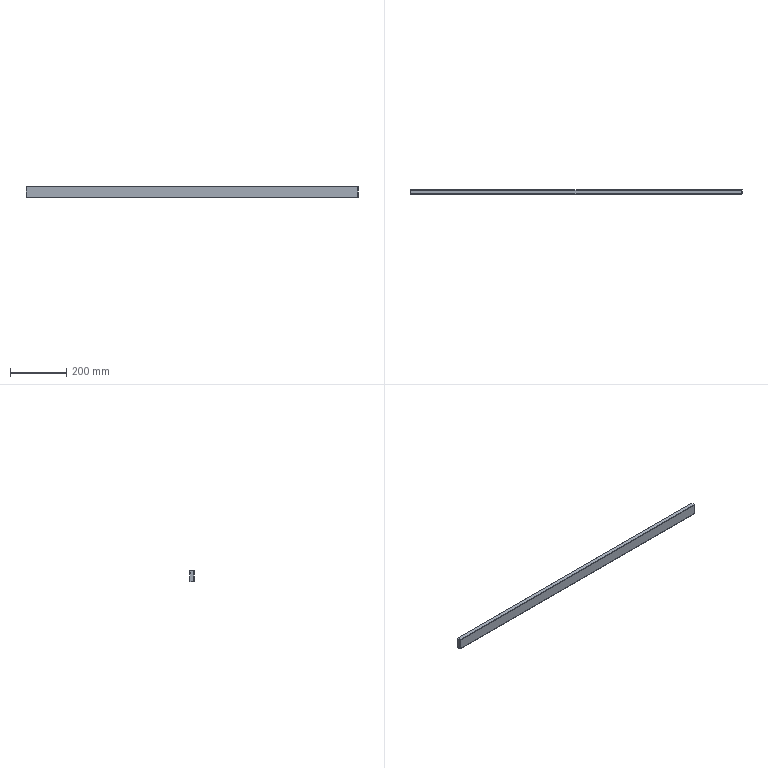Part | SolidWorks | features EdgeFlange 2, FlatPattern 1, SMBaseFlange 1, SheetMetal 1 | 1 solid | 46 faces | box 1180 x 15 x 40 mm | volume 107252 mm3 | plane 28 | cylinder 10 | spline 8 | commonest cylinder face diameters 0.9 x5 3.3 x5